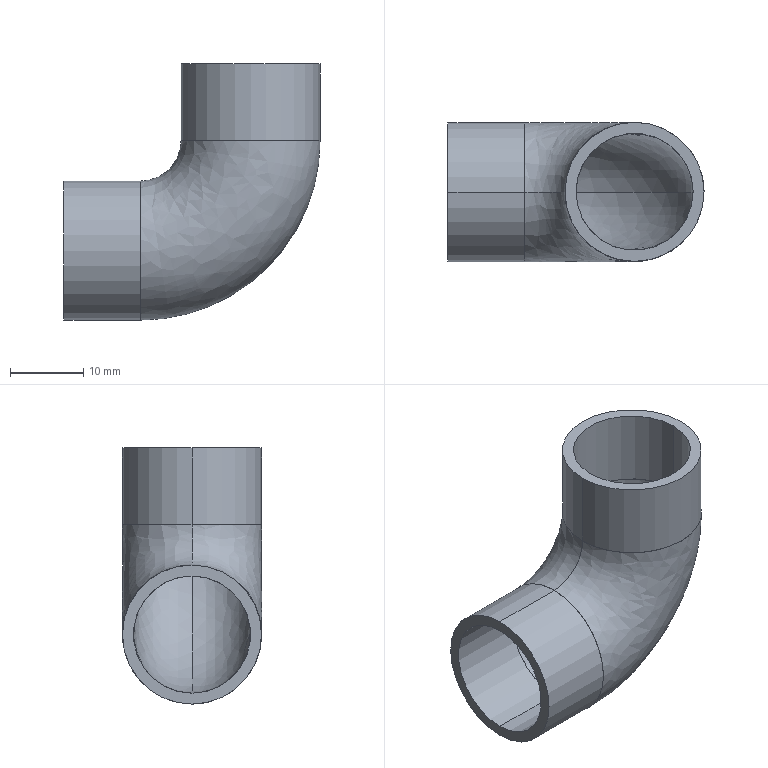Part | STEP file | three-quarters elbow_default_machined_ | 3 solids | 18 faces | box 35 x 19 x 35 mm | volume 3675 mm3 | cylinder 8 | plane 6 | spline 4 | commonest cylinder face diameters 16 x4 19 x4